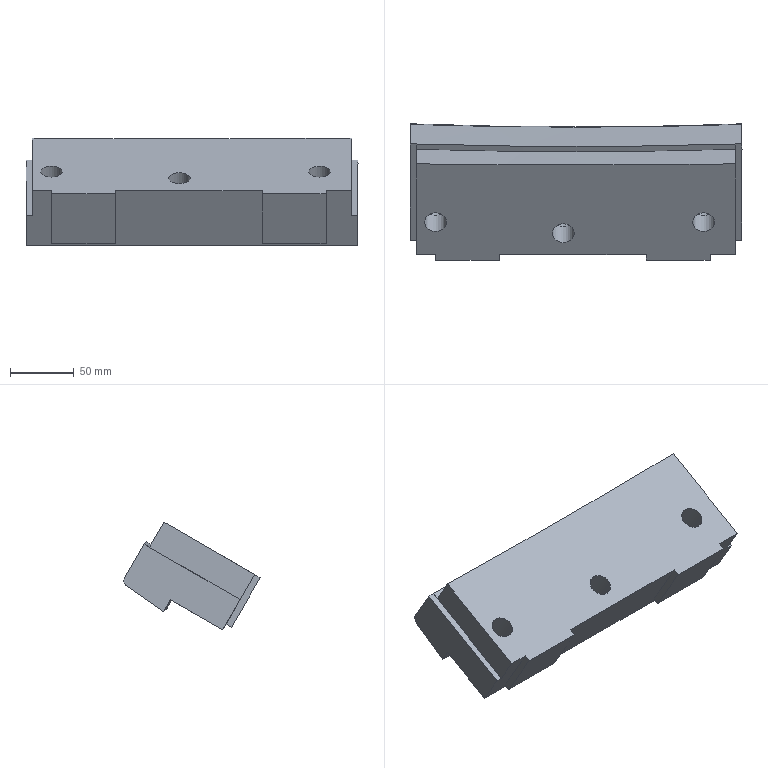Part | NX | features solid 2 | 1 solid | 36 faces | box 260 x 106.8 x 84.301 mm | volume 1120934 mm3 | plane 20 | spline 10 | cylinder 6 | commonest cylinder face diameters 17 x3 25 x3